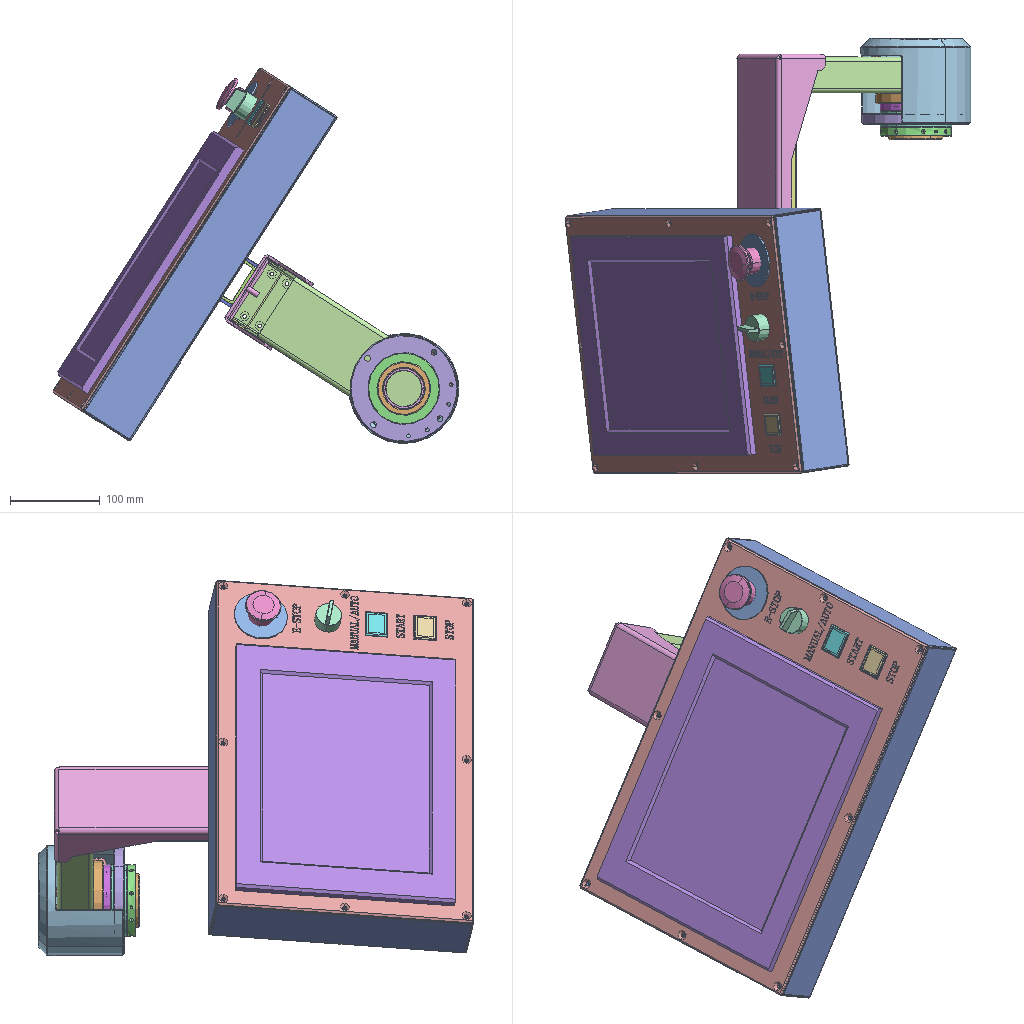Assembly | SolidWorks | 23 different items | 31 placed | box 453 x 486 x 419 mm
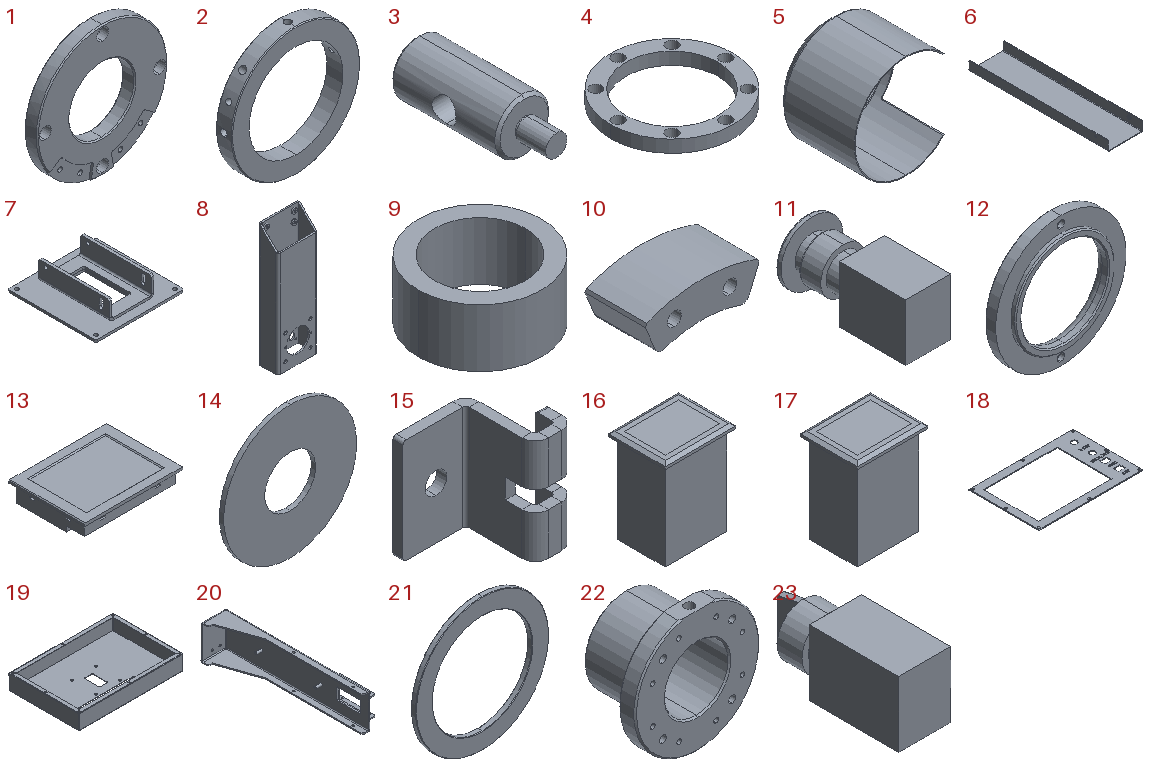Parts list (item | quantity | size | volume | features):
1 | x1 | 120 x 12 x 120 mm | 95094 mm3 | features HoleWzd 2, Chamfer 1, Extrusion 1, Fillet 1, ICE 1
2 | x1 | 80 x 10 x 80 mm | 22320 mm3 | features CirPattern 2, HoleWzd 2, Chamfer 1, Extrusion 1
3 | x4 | 10 x 26 x 10 mm | 1414 mm3 | features ICE 2, Chamfer 1, Extrusion 1, HoleWzd 1, RevCut 1
4 | x1 | 80 x 80 x 8 mm | 15493 mm3 | features CirPattern 1, Extrusion 1, HoleWzd 1
5 | x1 | 123 x 93.5 x 123 mm | 38171 mm3 | features Fillet 2, Chamfer 1, Extrusion 1, HoleWzd 1, ICE 1, Shell 1
6 | x1 | 81 x 325 x 21.5 mm | 58526 mm3 | features Chamfer 1, EdgeFlange 1, FlatPattern 1, HoleWzd 1, ICE 1, MirrorPattern 1, SMBaseFlange 1, SheetMetal 1
7 | x1 | 112 x 112 x 28 mm | 52364 mm3 | features Chamfer 2, FlatPattern 2, HoleWzd 2, ICE 2, SMBaseFlange 2, SheetMetal 2
8 | x1 | 80 x 40 x 245 mm | 145168 mm3 | features HoleWzd 5, ICE 4, Extrusion 1
9 | x1 | 17 x 17 x 8 mm | 834.093 mm3 | features Extrusion 1
10 | x2 | 45.157 x 24 x 16.667 mm | 11971 mm3 | features Chamfer 1, Extrusion 1, Fillet 1, HoleWzd 1, ICE 1
11 | x1 | 40 x 80 x 40 mm | 67108 mm3 | features ICE 4, Extrusion 1, Fillet 1, RevCut 1
12 | x1 | 60 x 7 x 60 mm | 7951 mm3 | features Chamfer 1, Extrusion 1, Fillet 1, HoleWzd 1, ICE 1
13 | x1 | 323 x 246 x 65.5 mm | 4046268 mm3 | features ICE 6, MirrorPattern 2, Chamfer 1, Extrusion 1
14 | x1 | 60 x 2 x 60 mm | 4824 mm3 | features Extrusion 1
15 | x4 | 15.5 x 12 x 15.8 mm | 586.671 mm3 | features Fillet 1, FlatPattern 1, HoleWzd 1, ICE 1, SMBaseFlange 1, SheetMetal 1
16 | x1 | 31 x 25 x 41 mm | 23593 mm3 | features Chamfer 1, Extrusion 1, ICE 1, PLine 1
17 | x1 | 31 x 25 x 41 mm | 23593 mm3 | features Chamfer 1, Extrusion 1, ICE 1, PLine 1
18 | x1 | 430 x 290 x 3 mm | 158728 mm3 | features ICE 4, Chamfer 1, Extrusion 1, HoleWzd 1
19 | x1 | 430 x 290 x 63 mm | 327890 mm3 | features ICE 4, SMWeldBead 4, EdgeFlange 2, HoleWzd 2, FlatPattern 1, SMBaseFlange 1, SheetMetal 1
20 | x1 | 83 x 363 x 88 mm | 165513 mm3 | features Chamfer 4, ICE 4, HoleWzd 3, FlatPattern 2, SMBaseFlange 2, SheetMetal 2, EdgeFlange 1
21 | x2 | 80 x 3 x 80 mm | 6558 mm3 | features Chamfer 1, Extrusion 1
22 | x1 | 90 x 52 x 88 mm | 99604 mm3 | features HoleWzd 3, ICE 3, Chamfer 1, CirPattern 1, Extrusion 1
23 | x1 | 29 x 80.3 x 36.6 mm | 65042 mm3 | features ICE 4, Extrusion 1, Fillet 1
Mates (type | each side: item.copy, entity, surface, feature):
Coincident | 18.1 face plane Boss-Extrude1 | 19.1 face plane Edge-Flange2
Coincident | 18.1 face plane Boss-Extrude1 | 19.1 face plane Edge-Flange1 | 2 times
Concentric | 21.1 face cylinder Boss-Extrude1 | 22.1 face cylinder Boss-Extrude2
Coincident | 21.1 face plane Boss-Extrude1 | 1.1 face plane Boss-Extrude1
Concentric | 22.1 face cylinder Boss-Extrude2 | 1.1 face cylinder Boss-Extrude1
Coincident | 1.1 face plane Boss-Extrude1 | 21.2 face plane Boss-Extrude1
Concentric | 22.1 face cylinder Boss-Extrude2 | 21.2 face cylinder Boss-Extrude1
Coincident | 21.2 face plane Boss-Extrude1 | 2.1 face plane Boss-Extrude1
Concentric | 22.1 face cylinder Boss-Extrude2 | 2.1 face cylinder Boss-Extrude1
Coincident | 20.1 face plane Base-Flange2 | 7.1 face plane Base-Flange2
Concentric | 20.1 face cylinder M4 Tapped Hole2 | 7.1 face cylinder Ø4.5 (4.5) Diameter Hole2
Concentric | 20.1 face cylinder M4 Tapped Hole2 | 7.1 face cylinder Cut-Extrude1
Concentric | 19.1 face cylinder M4 Tapped Hole2 | 7.1 face cylinder Ø4.5 (4.5) Diameter Hole1 | 2 times
Coincident | 19.1 face plane Base-Flange1 | 7.1 face plane Base-Flange1
Concentric | 22.1 face cylinder M6 Tapped Hole1 | 8.1 face cylinder Ø6.5 (6.5) Diameter Hole1 | 2 times
Coincident | 22.1 face plane Boss-Extrude1 | 8.1 face plane Boss-Extrude1
Coincident | 3.1 face plane Boss-Extrude1 | 8.1 face plane Boss-Extrude1
Coincident | 3.2 face plane Boss-Extrude1 | 3.1 face plane Boss-Extrude1
Coincident | 3.1 face plane Boss-Extrude1 | 3.3 face plane Boss-Extrude1
Coincident | 3.1 face plane Boss-Extrude1 | 3.4 face plane Boss-Extrude1
Concentric | 3.1 face cylinder Boss-Extrude1 | 8.1 face cylinder M4 Tapped Hole1
Concentric | 3.2 face cylinder Boss-Extrude1 | 8.1 face cylinder M4 Tapped Hole1
Concentric | 3.4 face cylinder Boss-Extrude1 | 8.1 face cylinder M4 Tapped Hole1
Concentric | 3.3 face cylinder Boss-Extrude1 | 8.1 face cylinder M4 Tapped Hole1
Concentric | 3.1 face cylinder Boss-Extrude1 | 5.1 face cylinder Ø4.5 (4.5) Diameter Hole1
Concentric | 3.4 face cylinder Boss-Extrude1 | 5.1 face cylinder Ø4.5 (4.5) Diameter Hole1
Width | 8.1 face plane Boss-Extrude1 | 8.1 face plane Boss-Extrude1 | 20.1 face plane Edge-Flange1 | 20.1 face plane Edge-Flange1
DistanceDim | 20.1 face plane Base-Flange1 | 8.1 face plane Boss-Extrude1
Coincident | 20.1 face plane Base-Flange1 | 8.1 face plane Boss-Extrude1
Coincident | 18.1 face plane Boss-Extrude1 | 11.1 face plane Boss-Extrude1
Concentric | 18.1 face cylinder Cut-Extrude2 | 11.1 face cylinder Boss-Extrude4
Coincident | 18.1 face plane Boss-Extrude1 | 23.1 face plane Boss-Extrude1
Concentric | 18.1 face cylinder Cut-Extrude2 | 23.1 face cylinder Boss-Extrude3
Width | 16.1 face plane Boss-Extrude1 | 16.1 face plane Boss-Extrude1 | 18.1 face plane Cut-Extrude3 | 18.1 face plane Cut-Extrude3
Width | 18.1 face plane Cut-Extrude3 | 18.1 face plane Cut-Extrude3 | 16.1 face plane Boss-Extrude1 | 16.1 face plane Boss-Extrude1
Coincident | 18.1 face plane Boss-Extrude1 | 16.1 face plane Boss-Extrude2
Width | 18.1 face plane Cut-Extrude3 | 18.1 face plane Cut-Extrude3 | 17.1 face plane Boss-Extrude1 | 17.1 face plane Boss-Extrude1
Width | 17.1 face plane Boss-Extrude1 | 17.1 face plane Boss-Extrude1 | 18.1 face plane Cut-Extrude3 | 18.1 face plane Cut-Extrude3
Coincident | 18.1 face plane Boss-Extrude1 | 17.1 face plane Boss-Extrude2
Width | 13.1 face plane Boss-Extrude1 | 13.1 face plane Boss-Extrude1 | 18.1 face plane Cut-Extrude1 | 18.1 face plane Cut-Extrude1
Width | 18.1 face plane Cut-Extrude1 | 18.1 face plane Cut-Extrude1 | 13.1 face plane Boss-Extrude1 | 13.1 face plane Boss-Extrude1
Coincident | 18.1 face plane Boss-Extrude1 | 13.1 face plane Boss-Extrude2
Concentric | 22.1 face cylinder Boss-Extrude2 | 4.1 face cylinder Boss-Extrude1
Coincident | 22.1 face plane Boss-Extrude1 | 4.1 face plane Boss-Extrude1
Coincident | 21.1 face plane Boss-Extrude1 | 4.1 face plane Boss-Extrude1
Coincident | 20.1 face plane Base-Flange1 | 6.1 face plane Edge-Flange1
Width | 20.1 face plane Edge-Flange1 | 20.1 face plane Edge-Flange1 | 6.1 face plane Edge-Flange1 | 6.1 face plane Edge-Flange1
DistanceDim | 6.1 face plane Edge-Flange1 | 20.1 face plane Base-Flange1
Coincident | 3.1 face plane Boss-Extrude1 | 5.1 face plane Shell1
Concentric | 22.1 face cylinder CirPattern1 | 4.1 face cylinder CirPattern1
Coincident | 22.1 face plane Cut-Extrude2 | 9.1 face plane Boss-Extrude1
Concentric | 1.1 face cylinder Boss-Extrude1 | 10.1 face cylinder Boss-Extrude1
Coincident | 1.1 face plane Cut-Extrude1 | 10.1 face plane Cut-Extrude1
Coincident | 1.1 face plane Cut-Extrude1 | 10.1 face plane Boss-Extrude1
Concentric | 1.1 face cylinder Boss-Extrude1 | 10.2 face cylinder Boss-Extrude1
Coincident | 1.1 face plane Cut-Extrude1 | 10.2 face plane Cut-Extrude1
Coincident | 1.1 face plane Cut-Extrude1 | 10.2 face plane Boss-Extrude1
Coincident | 18.1 face plane Boss-Extrude1 | 14.1 face plane Boss-Extrude1
Concentric | 11.1 face cylinder Boss-Extrude1 | 14.1 face cylinder Boss-Extrude1
Concentric | 22.1 face cylinder M8 Tapped Hole1 | 9.1 face cylinder Boss-Extrude1
Coincident | 13.1 face plane Mirror2 | 15.1 face plane Base-Flange1 | 2 times
Coincident | 13.1 face plane Boss-Extrude1 | 15.1 face plane Base-Flange1
Coincident | 13.1 face plane Boss-Extrude1 | 15.2 face plane Base-Flange1
Coincident | 13.1 face plane Cut-Extrude4 | 15.2 face plane Base-Flange1 | 2 times
Coincident | 13.1 face plane Mirror1 | 15.3 face plane Base-Flange1 | 2 times
Coincident | 13.1 face plane Boss-Extrude1 | 15.3 face plane Base-Flange1
Coincident | 13.1 face plane Boss-Extrude1 | 15.4 face plane Base-Flange1
Coincident | 13.1 face plane Cut-Extrude5 | 15.4 face plane Base-Flange1 | 2 times
Coincident | 8.1 face plane Boss-Extrude1 | 12.1 face plane Cut-Extrude1
Concentric | 22.1 face cylinder Cut-Extrude1 | 12.1 face cylinder Cut-Extrude1
Concentric | 8.1 face cylinder M3 Tapped Hole1 | 12.1 face cylinder Hole Size by Socket Head Cap Screw Type1